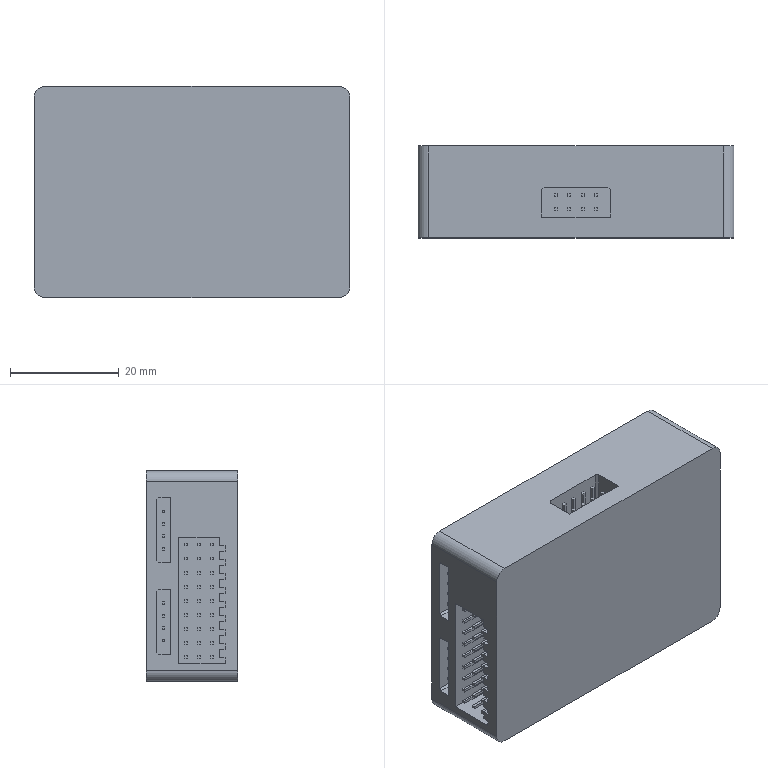Part | SolidWorks | features ICE 92, Chamfer 2, CenterOfMass 1, Extrusion 1, Fillet 1 | 1 solid | 556 faces | box 58.21 x 16.91 x 38.92 mm | volume 32464 mm3 | plane 552 | cylinder 4 | commonest cylinder face diameters 4 x4